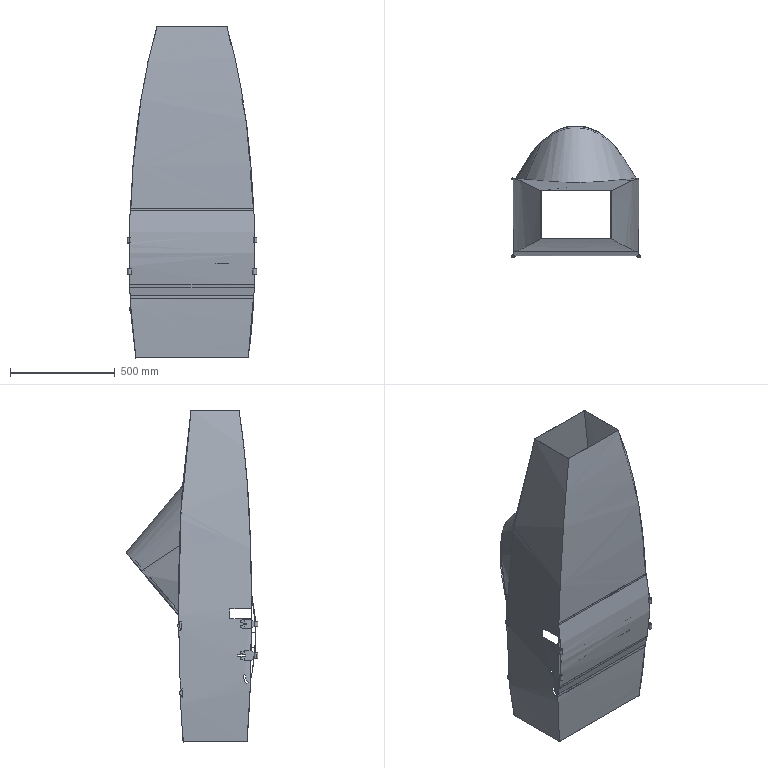Part | SolidWorks | features BaseBody 23 | 23 solids | 361 faces | box 618.426 x 629.876 x 1585 mm | volume 1303327 mm3 | plane 161 | cylinder 152 | spline 48 | commonest cylinder face diameters 3.2 x44 4.2 x32 7.765 x12 10 x12 6 x8 12 x8